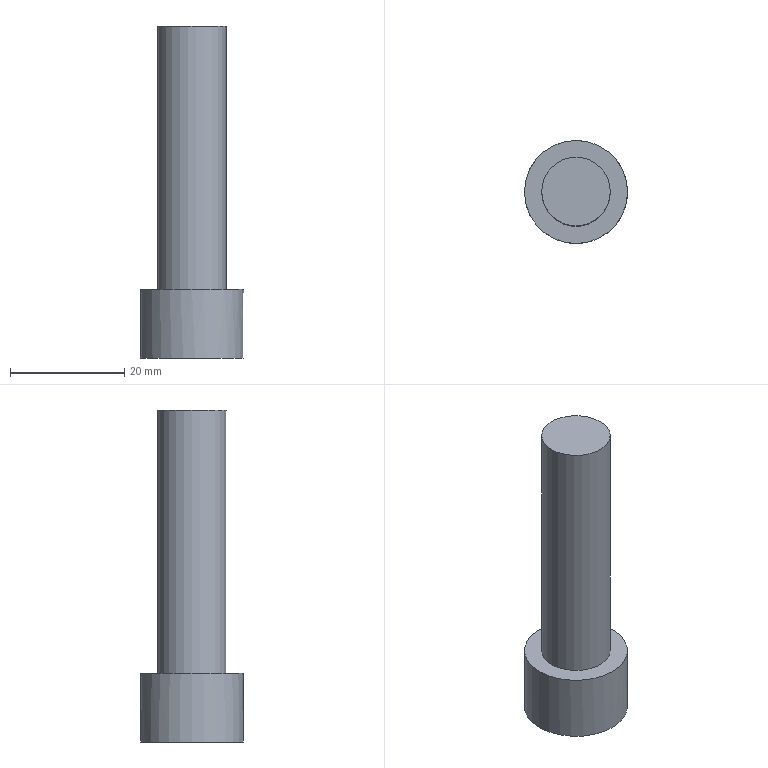Part | STEP file | solid 26 | 1 solid | 12 faces | box 18 x 18 x 58 mm | volume 7736 mm3 | plane 10 | cylinder 2 | commonest cylinder face diameters 12 x1 18 x1